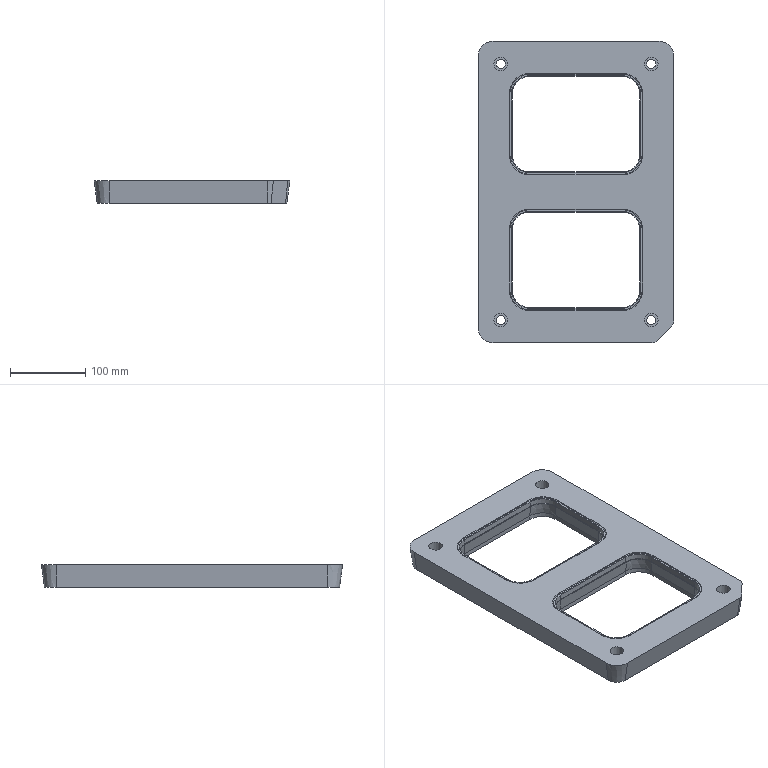Part | STEP file | SL2-MOLD_id650_xmt_txt | 1 solid | 108 faces | box 260 x 400 x 30 mm | volume 1707580 mm3 | plane 47 | cylinder 32 | cone 21 | torus 8 | commonest cylinder face diameters 1.829 x8 49.326 x8 54.458 x8 12 x4 18 x4